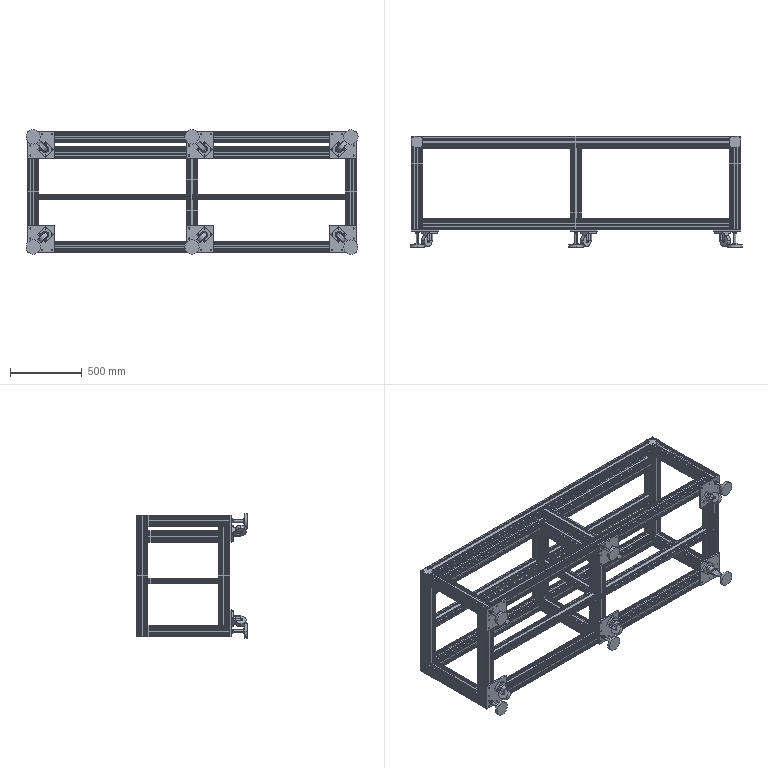Part | NX | 51 solids | 4150 faces | volume 49723378 mm3 | plane 3070 | cylinder 1008 | cone 72 | commonest cylinder face diameters 2 x304 6.8 x164 11.8 x108 8 x84 5.64 x72 6.75 x48